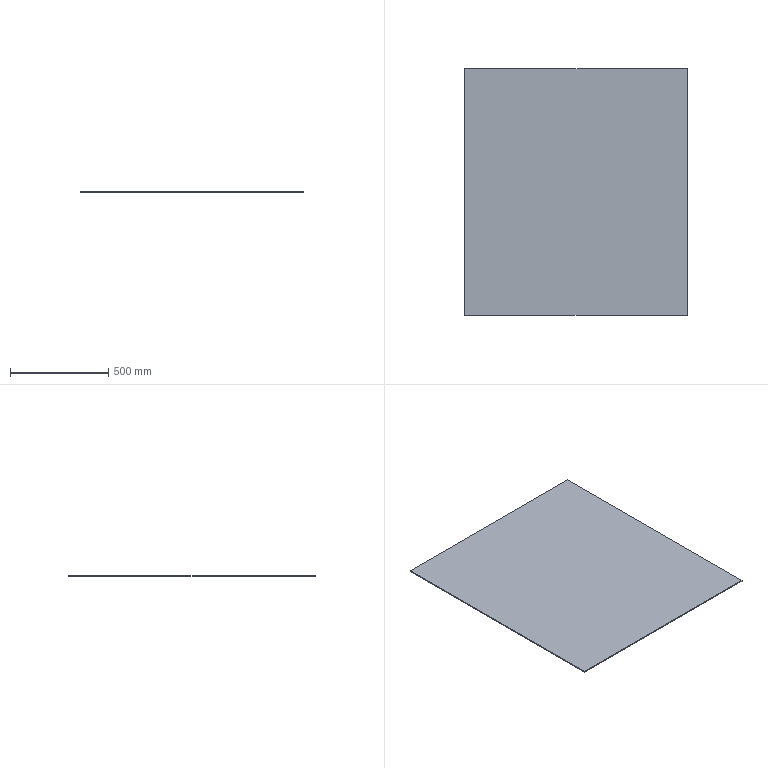Part | SolidWorks | features Extrusion 1 | 1 solid | 6 faces | box 1135 x 1255 x 5 mm | volume 7122125 mm3 | plane 6
STEP:
#1=CARTESIAN_POINT('',(567.5,-627.5,0.));
#2=VERTEX_POINT('',#1);
#3=CARTESIAN_POINT('',(567.5,627.5,0.));
#4=VERTEX_POINT('',#3);
#5=CARTESIAN_POINT('',(567.5,627.5,0.));
#6=DIRECTION('',(0.,1.,0.));
#7=VECTOR('',#6,1000.);
#8=LINE('',#5,#7);
#9=EDGE_CURVE('',#2,#4,#8,.T.);
#10=ORIENTED_EDGE('',*,*,#9,.T.);
#11=CARTESIAN_POINT('',(567.5,627.5,5.));
#12=VERTEX_POINT('',#11);
#13=CARTESIAN_POINT('',(567.5,627.5,5.));
#14=DIRECTION('',(0.,0.,-1.));
#15=VECTOR('',#14,1000.);
#16=LINE('',#13,#15);
#17=EDGE_CURVE('',#12,#4,#16,.T.);
#18=ORIENTED_EDGE('',*,*,#17,.F.);
#19=CARTESIAN_POINT('',(567.5,-627.5,5.));
#20=VERTEX_POINT('',#19);
#21=CARTESIAN_POINT('',(567.5,627.5,5.));
#22=DIRECTION('',(0.,1.,0.));
#23=VECTOR('',#22,1000.);
#24=LINE('',#21,#23);
#25=EDGE_CURVE('',#20,#12,#24,.T.);
#26=ORIENTED_EDGE('',*,*,#25,.F.);
#27=CARTESIAN_POINT('',(567.5,-627.5,5.));
#28=DIRECTION('',(0.,0.,-1.));
#29=VECTOR('',#28,1000.);
#30=LINE('',#27,#29);
#31=EDGE_CURVE('',#20,#2,#30,.T.);
#32=ORIENTED_EDGE('',*,*,#31,.T.);
#33=EDGE_LOOP('',(#10,#18,#26,#32));
#34=FACE_OUTER_BOUND('',#33,.T.);
#35=CARTESIAN_POINT('',(567.5,627.5,5.));
#36=DIRECTION('',(-1.,0.,0.));
#37=DIRECTION('',(0.,-1.,0.));
#38=AXIS2_PLACEMENT_3D('',#35,#36,#37);
#39=PLANE('',#38);
#40=ADVANCED_FACE('',(#34),#39,.F.);
#41=CARTESIAN_POINT('',(-567.5,627.5,0.));
#42=VERTEX_POINT('',#41);
#43=CARTESIAN_POINT('',(-567.5,627.5,0.));
#44=DIRECTION('',(-1.,0.,0.));
#45=VECTOR('',#44,1000.);
#46=LINE('',#43,#45);
#47=EDGE_CURVE('',#4,#42,#46,.T.);
#48=ORIENTED_EDGE('',*,*,#47,.T.);
#49=CARTESIAN_POINT('',(-567.5,627.5,5.));
#50=VERTEX_POINT('',#49);
#51=CARTESIAN_POINT('',(-567.5,627.5,5.));
#52=DIRECTION('',(0.,0.,-1.));
#53=VECTOR('',#52,1000.);
#54=LINE('',#51,#53);
#55=EDGE_CURVE('',#50,#42,#54,.T.);
#56=ORIENTED_EDGE('',*,*,#55,.F.);
#57=CARTESIAN_POINT('',(-567.5,627.5,5.));
#58=DIRECTION('',(-1.,0.,0.));
#59=VECTOR('',#58,1000.);
#60=LINE('',#57,#59);
#61=EDGE_CURVE('',#12,#50,#60,.T.);
#62=ORIENTED_EDGE('',*,*,#61,.F.);
#63=ORIENTED_EDGE('',*,*,#17,.T.);
#64=EDGE_LOOP('',(#48,#56,#62,#63));
#65=FACE_OUTER_BOUND('',#64,.T.);
#66=CARTESIAN_POINT('',(-567.5,627.5,5.));
#67=DIRECTION('',(0.,-1.,0.));
#68=DIRECTION('',(0.,0.,-1.));
#69=AXIS2_PLACEMENT_3D('',#66,#67,#68);
#70=PLANE('',#69);
#71=ADVANCED_FACE('',(#65),#70,.F.);
#72=CARTESIAN_POINT('',(-567.5,-627.5,0.));
#73=VERTEX_POINT('',#72);
#74=CARTESIAN_POINT('',(-567.5,627.5,0.));
#75=DIRECTION('',(0.,-1.,0.));
#76=VECTOR('',#75,1000.);
#77=LINE('',#74,#76);
#78=EDGE_CURVE('',#42,#73,#77,.T.);
#79=ORIENTED_EDGE('',*,*,#78,.T.);
#80=CARTESIAN_POINT('',(-567.5,-627.5,5.));
#81=VERTEX_POINT('',#80);
#82=CARTESIAN_POINT('',(-567.5,-627.5,5.));
#83=DIRECTION('',(0.,0.,-1.));
#84=VECTOR('',#83,1000.);
#85=LINE('',#82,#84);
#86=EDGE_CURVE('',#81,#73,#85,.T.);
#87=ORIENTED_EDGE('',*,*,#86,.F.);
#88=CARTESIAN_POINT('',(-567.5,627.5,5.));
#89=DIRECTION('',(0.,-1.,0.));
#90=VECTOR('',#89,1000.);
#91=LINE('',#88,#90);
#92=EDGE_CURVE('',#50,#81,#91,.T.);
#93=ORIENTED_EDGE('',*,*,#92,.F.);
#94=ORIENTED_EDGE('',*,*,#55,.T.);
#95=EDGE_LOOP('',(#79,#87,#93,#94));
#96=FACE_OUTER_BOUND('',#95,.T.);
#97=CARTESIAN_POINT('',(-567.5,627.5,5.));
#98=DIRECTION('',(1.,0.,0.));
#99=DIRECTION('',(0.,1.,0.));
#100=AXIS2_PLACEMENT_3D('',#97,#98,#99);
#101=PLANE('',#100);
#102=ADVANCED_FACE('',(#96),#101,.F.);
#103=CARTESIAN_POINT('',(-567.5,-627.5,0.));
#104=DIRECTION('',(1.,0.,0.));
#105=VECTOR('',#104,1000.);
#106=LINE('',#103,#105);
#107=EDGE_CURVE('',#73,#2,#106,.T.);
#108=ORIENTED_EDGE('',*,*,#107,.T.);
#109=ORIENTED_EDGE('',*,*,#31,.F.);
#110=CARTESIAN_POINT('',(-567.5,-627.5,5.));
#111=DIRECTION('',(1.,0.,0.));
#112=VECTOR('',#111,1000.);
#113=LINE('',#110,#112);
#114=EDGE_CURVE('',#81,#20,#113,.T.);
#115=ORIENTED_EDGE('',*,*,#114,.F.);
#116=ORIENTED_EDGE('',*,*,#86,.T.);
#117=EDGE_LOOP('',(#108,#109,#115,#116));
#118=FACE_OUTER_BOUND('',#117,.T.);
#119=CARTESIAN_POINT('',(-567.5,-627.5,5.));
#120=DIRECTION('',(0.,1.,0.));
#121=DIRECTION('',(0.,0.,1.));
#122=AXIS2_PLACEMENT_3D('',#119,#120,#121);
#123=PLANE('',#122);
#124=ADVANCED_FACE('',(#118),#123,.F.);
#125=ORIENTED_EDGE('',*,*,#25,.T.);
#126=ORIENTED_EDGE('',*,*,#61,.T.);
#127=ORIENTED_EDGE('',*,*,#92,.T.);
#128=ORIENTED_EDGE('',*,*,#114,.T.);
#129=EDGE_LOOP('',(#125,#126,#127,#128));
#130=FACE_OUTER_BOUND('',#129,.T.);
#131=CARTESIAN_POINT('',(0.,0.,5.));
#132=DIRECTION('',(0.,0.,1.));
#133=DIRECTION('',(1.,0.,0.));
#134=AXIS2_PLACEMENT_3D('',#131,#132,#133);
#135=PLANE('',#134);
#136=ADVANCED_FACE('',(#130),#135,.T.);
#137=ORIENTED_EDGE('',*,*,#9,.F.);
#138=ORIENTED_EDGE('',*,*,#107,.F.);
#139=ORIENTED_EDGE('',*,*,#78,.F.);
#140=ORIENTED_EDGE('',*,*,#47,.F.);
#141=EDGE_LOOP('',(#137,#138,#139,#140));
#142=FACE_OUTER_BOUND('',#141,.T.);
#143=CARTESIAN_POINT('',(0.,0.,0.));
#144=DIRECTION('',(0.,0.,1.));
#145=DIRECTION('',(1.,0.,0.));
#146=AXIS2_PLACEMENT_3D('',#143,#144,#145);
#147=PLANE('',#146);
#148=ADVANCED_FACE('',(#142),#147,.F.);
#149=CLOSED_SHELL('',(#40,#71,#102,#124,#136,#148));
#150=MANIFOLD_SOLID_BREP('',#149);
#151=CARTESIAN_POINT('',(0.,0.,0.));
#152=DIRECTION('',(0.,0.,1.));
#153=DIRECTION('',(1.,0.,0.));
#154=AXIS2_PLACEMENT_3D('',#151,#152,#153);
#155=(LENGTH_UNIT()NAMED_UNIT(*)SI_UNIT(.MILLI.,.METRE.));
#156=UNCERTAINTY_MEASURE_WITH_UNIT(LENGTH_MEASURE(0.00001),#155,'','');
#157=(NAMED_UNIT(*)PLANE_ANGLE_UNIT()SI_UNIT($,.RADIAN.));
#158=(NAMED_UNIT(*)SI_UNIT($,.STERADIAN.)SOLID_ANGLE_UNIT());
#159=(GEOMETRIC_REPRESENTATION_CONTEXT(3)GLOBAL_UNCERTAINTY_ASSIGNED_CONTEXT((#156))GLOBAL_UNIT_ASSIGNED_CONTEXT((#155,#157,#158))REPRESENTATION_CONTEXT('',''));
#160=ADVANCED_BREP_SHAPE_REPRESENTATION('',(#150,#154),#159);